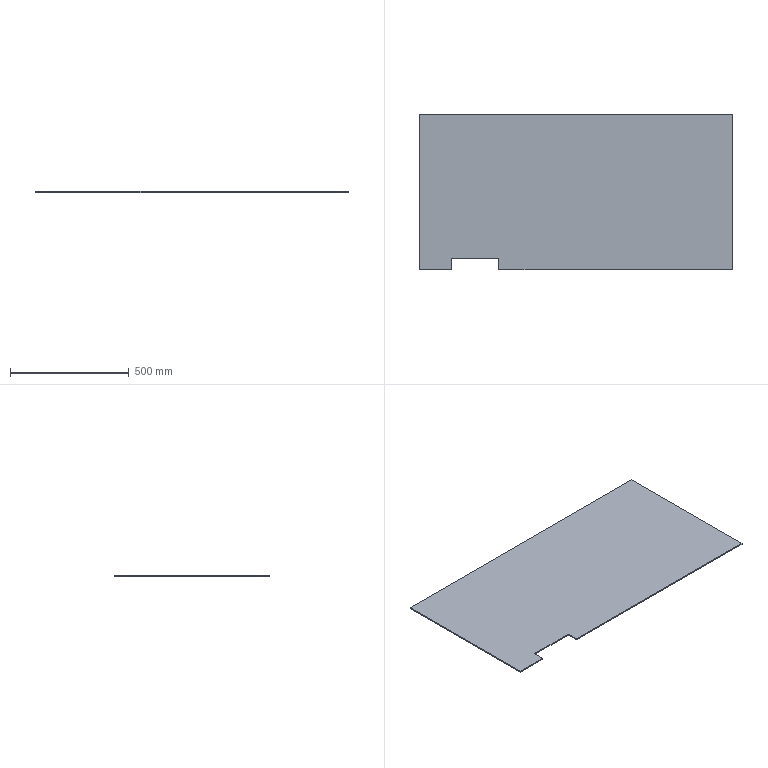Part | STEP file | 1 solid | 10 faces | box 1318 x 655 x 5 mm | volume 4267450 mm3 | plane 10
STEP:
#1=CARTESIAN_POINT('',(0.,0.,0.));
#2=DIRECTION('',(0.,0.,1.));
#3=DIRECTION('',(1.,0.,0.));
#4=AXIS2_PLACEMENT_3D('',#1,#2,#3);
#5=CARTESIAN_POINT('',(-324.,-657.,0.));
#6=VERTEX_POINT('',#5);
#7=CARTESIAN_POINT('',(-524.,-657.,0.));
#8=VERTEX_POINT('',#7);
#9=CARTESIAN_POINT('',(-524.,-657.,0.));
#10=DIRECTION('',(-1.,0.,0.));
#11=VECTOR('',#10,1.);
#12=LINE('',#9,#11);
#13=CARTESIAN_POINT('',(0.,0.,0.));
#14=DIRECTION('',(0.,0.,1.));
#15=DIRECTION('',(1.,0.,0.));
#16=AXIS2_PLACEMENT_3D('',#13,#14,#15);
#17=PLANE('',#16);
#18=CARTESIAN_POINT('',(-524.,-657.));
#19=DIRECTION('',(-1.,0.));
#20=VECTOR('',#19,1.);
#21=LINE('',#18,#20);
#22=(GEOMETRIC_REPRESENTATION_CONTEXT(2)PARAMETRIC_REPRESENTATION_CONTEXT()REPRESENTATION_CONTEXT('',''));
#23=DEFINITIONAL_REPRESENTATION('',(#21),#22);
#24=PCURVE('',#17,#23);
#25=CARTESIAN_POINT('',(-524.,-657.,5.));
#26=DIRECTION('',(0.,1.,0.));
#27=DIRECTION('',(1.,0.,0.));
#28=AXIS2_PLACEMENT_3D('',#25,#26,#27);
#29=PLANE('',#28);
#30=CARTESIAN_POINT('',(0.,5.));
#31=DIRECTION('',(-1.,0.));
#32=VECTOR('',#31,1.);
#33=LINE('',#30,#32);
#34=(GEOMETRIC_REPRESENTATION_CONTEXT(2)PARAMETRIC_REPRESENTATION_CONTEXT()REPRESENTATION_CONTEXT('',''));
#35=DEFINITIONAL_REPRESENTATION('',(#33),#34);
#36=PCURVE('',#29,#35);
#37=SURFACE_CURVE('',#12,(#24,#36),.PCURVE_S1.);
#38=EDGE_CURVE('',#6,#8,#37,.T.);
#39=ORIENTED_EDGE('',*,*,#38,.T.);
#40=CARTESIAN_POINT('',(-524.,-706.,0.));
#41=VERTEX_POINT('',#40);
#42=CARTESIAN_POINT('',(-524.,-657.,0.));
#43=DIRECTION('',(0.,1.,0.));
#44=VECTOR('',#43,1.);
#45=LINE('',#42,#44);
#46=CARTESIAN_POINT('',(-524.,-657.));
#47=DIRECTION('',(0.,1.));
#48=VECTOR('',#47,1.);
#49=LINE('',#46,#48);
#50=(GEOMETRIC_REPRESENTATION_CONTEXT(2)PARAMETRIC_REPRESENTATION_CONTEXT()REPRESENTATION_CONTEXT('',''));
#51=DEFINITIONAL_REPRESENTATION('',(#49),#50);
#52=PCURVE('',#17,#51);
#53=CARTESIAN_POINT('',(-524.,-657.,5.));
#54=DIRECTION('',(1.,0.,0.));
#55=DIRECTION('',(0.,1.,0.));
#56=AXIS2_PLACEMENT_3D('',#53,#54,#55);
#57=PLANE('',#56);
#58=CARTESIAN_POINT('',(0.,-5.));
#59=DIRECTION('',(1.,0.));
#60=VECTOR('',#59,1.);
#61=LINE('',#58,#60);
#62=(GEOMETRIC_REPRESENTATION_CONTEXT(2)PARAMETRIC_REPRESENTATION_CONTEXT()REPRESENTATION_CONTEXT('',''));
#63=DEFINITIONAL_REPRESENTATION('',(#61),#62);
#64=PCURVE('',#57,#63);
#65=SURFACE_CURVE('',#45,(#52,#64),.PCURVE_S1.);
#66=EDGE_CURVE('',#41,#8,#65,.T.);
#67=ORIENTED_EDGE('',*,*,#66,.F.);
#68=CARTESIAN_POINT('',(-659.,-706.,0.));
#69=VERTEX_POINT('',#68);
#70=CARTESIAN_POINT('',(-659.,-706.,0.));
#71=DIRECTION('',(-1.,0.,0.));
#72=VECTOR('',#71,1.);
#73=LINE('',#70,#72);
#74=CARTESIAN_POINT('',(-659.,-706.));
#75=DIRECTION('',(-1.,0.));
#76=VECTOR('',#75,1.);
#77=LINE('',#74,#76);
#78=(GEOMETRIC_REPRESENTATION_CONTEXT(2)PARAMETRIC_REPRESENTATION_CONTEXT()REPRESENTATION_CONTEXT('',''));
#79=DEFINITIONAL_REPRESENTATION('',(#77),#78);
#80=PCURVE('',#17,#79);
#81=CARTESIAN_POINT('',(-659.,-706.,5.));
#82=DIRECTION('',(0.,1.,0.));
#83=DIRECTION('',(1.,0.,0.));
#84=AXIS2_PLACEMENT_3D('',#81,#82,#83);
#85=PLANE('',#84);
#86=CARTESIAN_POINT('',(0.,5.));
#87=DIRECTION('',(-1.,0.));
#88=VECTOR('',#87,1.);
#89=LINE('',#86,#88);
#90=(GEOMETRIC_REPRESENTATION_CONTEXT(2)PARAMETRIC_REPRESENTATION_CONTEXT()REPRESENTATION_CONTEXT('',''));
#91=DEFINITIONAL_REPRESENTATION('',(#89),#90);
#92=PCURVE('',#85,#91);
#93=SURFACE_CURVE('',#73,(#80,#92),.PCURVE_S1.);
#94=EDGE_CURVE('',#41,#69,#93,.T.);
#95=ORIENTED_EDGE('',*,*,#94,.T.);
#96=CARTESIAN_POINT('',(-659.,-51.,0.));
#97=VERTEX_POINT('',#96);
#98=CARTESIAN_POINT('',(-659.,-51.,0.));
#99=DIRECTION('',(0.,1.,0.));
#100=VECTOR('',#99,1.);
#101=LINE('',#98,#100);
#102=CARTESIAN_POINT('',(-659.,-51.));
#103=DIRECTION('',(0.,1.));
#104=VECTOR('',#103,1.);
#105=LINE('',#102,#104);
#106=(GEOMETRIC_REPRESENTATION_CONTEXT(2)PARAMETRIC_REPRESENTATION_CONTEXT()REPRESENTATION_CONTEXT('',''));
#107=DEFINITIONAL_REPRESENTATION('',(#105),#106);
#108=PCURVE('',#17,#107);
#109=CARTESIAN_POINT('',(-659.,-51.,5.));
#110=DIRECTION('',(1.,0.,0.));
#111=DIRECTION('',(0.,1.,0.));
#112=AXIS2_PLACEMENT_3D('',#109,#110,#111);
#113=PLANE('',#112);
#114=CARTESIAN_POINT('',(0.,-5.));
#115=DIRECTION('',(1.,0.));
#116=VECTOR('',#115,1.);
#117=LINE('',#114,#116);
#118=(GEOMETRIC_REPRESENTATION_CONTEXT(2)PARAMETRIC_REPRESENTATION_CONTEXT()REPRESENTATION_CONTEXT('',''));
#119=DEFINITIONAL_REPRESENTATION('',(#117),#118);
#120=PCURVE('',#113,#119);
#121=SURFACE_CURVE('',#101,(#108,#120),.PCURVE_S1.);
#122=EDGE_CURVE('',#69,#97,#121,.T.);
#123=ORIENTED_EDGE('',*,*,#122,.T.);
#124=CARTESIAN_POINT('',(659.,-51.,0.));
#125=VERTEX_POINT('',#124);
#126=CARTESIAN_POINT('',(-659.,-51.,0.));
#127=DIRECTION('',(-1.,0.,0.));
#128=VECTOR('',#127,1.);
#129=LINE('',#126,#128);
#130=CARTESIAN_POINT('',(-659.,-51.));
#131=DIRECTION('',(-1.,0.));
#132=VECTOR('',#131,1.);
#133=LINE('',#130,#132);
#134=(GEOMETRIC_REPRESENTATION_CONTEXT(2)PARAMETRIC_REPRESENTATION_CONTEXT()REPRESENTATION_CONTEXT('',''));
#135=DEFINITIONAL_REPRESENTATION('',(#133),#134);
#136=PCURVE('',#17,#135);
#137=CARTESIAN_POINT('',(-659.,-51.,5.));
#138=DIRECTION('',(0.,1.,0.));
#139=DIRECTION('',(1.,0.,0.));
#140=AXIS2_PLACEMENT_3D('',#137,#138,#139);
#141=PLANE('',#140);
#142=CARTESIAN_POINT('',(0.,5.));
#143=DIRECTION('',(-1.,0.));
#144=VECTOR('',#143,1.);
#145=LINE('',#142,#144);
#146=(GEOMETRIC_REPRESENTATION_CONTEXT(2)PARAMETRIC_REPRESENTATION_CONTEXT()REPRESENTATION_CONTEXT('',''));
#147=DEFINITIONAL_REPRESENTATION('',(#145),#146);
#148=PCURVE('',#141,#147);
#149=SURFACE_CURVE('',#129,(#136,#148),.PCURVE_S1.);
#150=EDGE_CURVE('',#125,#97,#149,.T.);
#151=ORIENTED_EDGE('',*,*,#150,.F.);
#152=CARTESIAN_POINT('',(659.,-706.,0.));
#153=VERTEX_POINT('',#152);
#154=CARTESIAN_POINT('',(659.,-51.,0.));
#155=DIRECTION('',(0.,1.,0.));
#156=VECTOR('',#155,1.);
#157=LINE('',#154,#156);
#158=CARTESIAN_POINT('',(659.,-51.));
#159=DIRECTION('',(0.,1.));
#160=VECTOR('',#159,1.);
#161=LINE('',#158,#160);
#162=(GEOMETRIC_REPRESENTATION_CONTEXT(2)PARAMETRIC_REPRESENTATION_CONTEXT()REPRESENTATION_CONTEXT('',''));
#163=DEFINITIONAL_REPRESENTATION('',(#161),#162);
#164=PCURVE('',#17,#163);
#165=CARTESIAN_POINT('',(659.,-51.,5.));
#166=DIRECTION('',(1.,0.,0.));
#167=DIRECTION('',(0.,1.,0.));
#168=AXIS2_PLACEMENT_3D('',#165,#166,#167);
#169=PLANE('',#168);
#170=CARTESIAN_POINT('',(0.,-5.));
#171=DIRECTION('',(1.,0.));
#172=VECTOR('',#171,1.);
#173=LINE('',#170,#172);
#174=(GEOMETRIC_REPRESENTATION_CONTEXT(2)PARAMETRIC_REPRESENTATION_CONTEXT()REPRESENTATION_CONTEXT('',''));
#175=DEFINITIONAL_REPRESENTATION('',(#173),#174);
#176=PCURVE('',#169,#175);
#177=SURFACE_CURVE('',#157,(#164,#176),.PCURVE_S1.);
#178=EDGE_CURVE('',#153,#125,#177,.T.);
#179=ORIENTED_EDGE('',*,*,#178,.F.);
#180=CARTESIAN_POINT('',(-324.,-706.,0.));
#181=VERTEX_POINT('',#180);
#182=CARTESIAN_POINT('',(-324.,-706.,0.));
#183=DIRECTION('',(-1.,0.,0.));
#184=VECTOR('',#183,1.);
#185=LINE('',#182,#184);
#186=CARTESIAN_POINT('',(-324.,-706.));
#187=DIRECTION('',(-1.,0.));
#188=VECTOR('',#187,1.);
#189=LINE('',#186,#188);
#190=(GEOMETRIC_REPRESENTATION_CONTEXT(2)PARAMETRIC_REPRESENTATION_CONTEXT()REPRESENTATION_CONTEXT('',''));
#191=DEFINITIONAL_REPRESENTATION('',(#189),#190);
#192=PCURVE('',#17,#191);
#193=CARTESIAN_POINT('',(-324.,-706.,5.));
#194=DIRECTION('',(0.,1.,0.));
#195=DIRECTION('',(1.,0.,0.));
#196=AXIS2_PLACEMENT_3D('',#193,#194,#195);
#197=PLANE('',#196);
#198=CARTESIAN_POINT('',(0.,5.));
#199=DIRECTION('',(-1.,0.));
#200=VECTOR('',#199,1.);
#201=LINE('',#198,#200);
#202=(GEOMETRIC_REPRESENTATION_CONTEXT(2)PARAMETRIC_REPRESENTATION_CONTEXT()REPRESENTATION_CONTEXT('',''));
#203=DEFINITIONAL_REPRESENTATION('',(#201),#202);
#204=PCURVE('',#197,#203);
#205=SURFACE_CURVE('',#185,(#192,#204),.PCURVE_S1.);
#206=EDGE_CURVE('',#153,#181,#205,.T.);
#207=ORIENTED_EDGE('',*,*,#206,.T.);
#208=CARTESIAN_POINT('',(-324.,-657.,0.));
#209=DIRECTION('',(0.,1.,0.));
#210=VECTOR('',#209,1.);
#211=LINE('',#208,#210);
#212=CARTESIAN_POINT('',(-324.,-657.));
#213=DIRECTION('',(0.,1.));
#214=VECTOR('',#213,1.);
#215=LINE('',#212,#214);
#216=(GEOMETRIC_REPRESENTATION_CONTEXT(2)PARAMETRIC_REPRESENTATION_CONTEXT()REPRESENTATION_CONTEXT('',''));
#217=DEFINITIONAL_REPRESENTATION('',(#215),#216);
#218=PCURVE('',#17,#217);
#219=CARTESIAN_POINT('',(-324.,-657.,5.));
#220=DIRECTION('',(1.,0.,0.));
#221=DIRECTION('',(0.,-1.,0.));
#222=AXIS2_PLACEMENT_3D('',#219,#220,#221);
#223=PLANE('',#222);
#224=CARTESIAN_POINT('',(0.,5.));
#225=DIRECTION('',(-1.,0.));
#226=VECTOR('',#225,1.);
#227=LINE('',#224,#226);
#228=(GEOMETRIC_REPRESENTATION_CONTEXT(2)PARAMETRIC_REPRESENTATION_CONTEXT()REPRESENTATION_CONTEXT('',''));
#229=DEFINITIONAL_REPRESENTATION('',(#227),#228);
#230=PCURVE('',#223,#229);
#231=SURFACE_CURVE('',#211,(#218,#230),.PCURVE_S1.);
#232=EDGE_CURVE('',#181,#6,#231,.T.);
#233=ORIENTED_EDGE('',*,*,#232,.T.);
#234=EDGE_LOOP('',(#39,#67,#95,#123,#151,#179,#207,#233));
#235=FACE_BOUND('',#234,.T.);
#236=ADVANCED_FACE('',(#235),#17,.F.);
#237=CARTESIAN_POINT('',(-324.,-706.,5.));
#238=VERTEX_POINT('',#237);
#239=CARTESIAN_POINT('',(-324.,-706.,5.));
#240=DIRECTION('',(0.,0.,1.));
#241=VECTOR('',#240,1.);
#242=LINE('',#239,#241);
#243=CARTESIAN_POINT('',(49.,0.));
#244=DIRECTION('',(0.,-1.));
#245=VECTOR('',#244,1.);
#246=LINE('',#243,#245);
#247=(GEOMETRIC_REPRESENTATION_CONTEXT(2)PARAMETRIC_REPRESENTATION_CONTEXT()REPRESENTATION_CONTEXT('',''));
#248=DEFINITIONAL_REPRESENTATION('',(#246),#247);
#249=PCURVE('',#223,#248);
#250=CARTESIAN_POINT('',(0.,0.));
#251=DIRECTION('',(0.,-1.));
#252=VECTOR('',#251,1.);
#253=LINE('',#250,#252);
#254=(GEOMETRIC_REPRESENTATION_CONTEXT(2)PARAMETRIC_REPRESENTATION_CONTEXT()REPRESENTATION_CONTEXT('',''));
#255=DEFINITIONAL_REPRESENTATION('',(#253),#254);
#256=PCURVE('',#197,#255);
#257=SURFACE_CURVE('',#242,(#249,#256),.PCURVE_S1.);
#258=EDGE_CURVE('',#181,#238,#257,.T.);
#259=ORIENTED_EDGE('',*,*,#258,.T.);
#260=CARTESIAN_POINT('',(-324.,-657.,5.));
#261=VERTEX_POINT('',#260);
#262=CARTESIAN_POINT('',(-324.,0.,5.));
#263=DIRECTION('',(0.,-1.,0.));
#264=VECTOR('',#263,1.);
#265=LINE('',#262,#264);
#266=CARTESIAN_POINT('',(-657.,0.));
#267=DIRECTION('',(1.,0.));
#268=VECTOR('',#267,1.);
#269=LINE('',#266,#268);
#270=(GEOMETRIC_REPRESENTATION_CONTEXT(2)PARAMETRIC_REPRESENTATION_CONTEXT()REPRESENTATION_CONTEXT('',''));
#271=DEFINITIONAL_REPRESENTATION('',(#269),#270);
#272=PCURVE('',#223,#271);
#273=CARTESIAN_POINT('',(0.,0.,5.));
#274=DIRECTION('',(0.,0.,1.));
#275=DIRECTION('',(1.,0.,0.));
#276=AXIS2_PLACEMENT_3D('',#273,#274,#275);
#277=PLANE('',#276);
#278=CARTESIAN_POINT('',(-324.,0.));
#279=DIRECTION('',(0.,-1.));
#280=VECTOR('',#279,1.);
#281=LINE('',#278,#280);
#282=(GEOMETRIC_REPRESENTATION_CONTEXT(2)PARAMETRIC_REPRESENTATION_CONTEXT()REPRESENTATION_CONTEXT('',''));
#283=DEFINITIONAL_REPRESENTATION('',(#281),#282);
#284=PCURVE('',#277,#283);
#285=SURFACE_CURVE('',#265,(#272,#284),.PCURVE_S1.);
#286=EDGE_CURVE('',#261,#238,#285,.T.);
#287=ORIENTED_EDGE('',*,*,#286,.F.);
#288=CARTESIAN_POINT('',(-324.,-657.,5.));
#289=DIRECTION('',(0.,0.,-1.));
#290=VECTOR('',#289,1.);
#291=LINE('',#288,#290);
#292=CARTESIAN_POINT('',(0.,0.));
#293=DIRECTION('',(0.,1.));
#294=VECTOR('',#293,1.);
#295=LINE('',#292,#294);
#296=(GEOMETRIC_REPRESENTATION_CONTEXT(2)PARAMETRIC_REPRESENTATION_CONTEXT()REPRESENTATION_CONTEXT('',''));
#297=DEFINITIONAL_REPRESENTATION('',(#295),#296);
#298=PCURVE('',#223,#297);
#299=CARTESIAN_POINT('',(200.,0.));
#300=DIRECTION('',(0.,1.));
#301=VECTOR('',#300,1.);
#302=LINE('',#299,#301);
#303=(GEOMETRIC_REPRESENTATION_CONTEXT(2)PARAMETRIC_REPRESENTATION_CONTEXT()REPRESENTATION_CONTEXT('',''));
#304=DEFINITIONAL_REPRESENTATION('',(#302),#303);
#305=PCURVE('',#29,#304);
#306=SURFACE_CURVE('',#291,(#298,#305),.PCURVE_S1.);
#307=EDGE_CURVE('',#261,#6,#306,.T.);
#308=ORIENTED_EDGE('',*,*,#307,.T.);
#309=ORIENTED_EDGE('',*,*,#232,.F.);
#310=EDGE_LOOP('',(#259,#287,#308,#309));
#311=FACE_BOUND('',#310,.T.);
#312=ADVANCED_FACE('',(#311),#223,.F.);
#313=CARTESIAN_POINT('',(659.,-706.,5.));
#314=VERTEX_POINT('',#313);
#315=CARTESIAN_POINT('',(659.,-706.,5.));
#316=DIRECTION('',(0.,0.,-1.));
#317=VECTOR('',#316,1.);
#318=LINE('',#315,#317);
#319=CARTESIAN_POINT('',(983.,0.));
#320=DIRECTION('',(0.,1.));
#321=VECTOR('',#320,1.);
#322=LINE('',#319,#321);
#323=(GEOMETRIC_REPRESENTATION_CONTEXT(2)PARAMETRIC_REPRESENTATION_CONTEXT()REPRESENTATION_CONTEXT('',''));
#324=DEFINITIONAL_REPRESENTATION('',(#322),#323);
#325=PCURVE('',#197,#324);
#326=CARTESIAN_POINT('',(-655.,0.));
#327=DIRECTION('',(0.,-1.));
#328=VECTOR('',#327,1.);
#329=LINE('',#326,#328);
#330=(GEOMETRIC_REPRESENTATION_CONTEXT(2)PARAMETRIC_REPRESENTATION_CONTEXT()REPRESENTATION_CONTEXT('',''));
#331=DEFINITIONAL_REPRESENTATION('',(#329),#330);
#332=PCURVE('',#169,#331);
#333=SURFACE_CURVE('',#318,(#325,#332),.PCURVE_S1.);
#334=EDGE_CURVE('',#314,#153,#333,.T.);
#335=ORIENTED_EDGE('',*,*,#334,.F.);
#336=CARTESIAN_POINT('',(0.,-706.,5.));
#337=DIRECTION('',(1.,0.,0.));
#338=VECTOR('',#337,1.);
#339=LINE('',#336,#338);
#340=CARTESIAN_POINT('',(324.,0.));
#341=DIRECTION('',(1.,0.));
#342=VECTOR('',#341,1.);
#343=LINE('',#340,#342);
#344=(GEOMETRIC_REPRESENTATION_CONTEXT(2)PARAMETRIC_REPRESENTATION_CONTEXT()REPRESENTATION_CONTEXT('',''));
#345=DEFINITIONAL_REPRESENTATION('',(#343),#344);
#346=PCURVE('',#197,#345);
#347=CARTESIAN_POINT('',(0.,-706.));
#348=DIRECTION('',(1.,0.));
#349=VECTOR('',#348,1.);
#350=LINE('',#347,#349);
#351=(GEOMETRIC_REPRESENTATION_CONTEXT(2)PARAMETRIC_REPRESENTATION_CONTEXT()REPRESENTATION_CONTEXT('',''));
#352=DEFINITIONAL_REPRESENTATION('',(#350),#351);
#353=PCURVE('',#277,#352);
#354=SURFACE_CURVE('',#339,(#346,#353),.PCURVE_S1.);
#355=EDGE_CURVE('',#238,#314,#354,.T.);
#356=ORIENTED_EDGE('',*,*,#355,.F.);
#357=ORIENTED_EDGE('',*,*,#258,.F.);
#358=ORIENTED_EDGE('',*,*,#206,.F.);
#359=EDGE_LOOP('',(#335,#356,#357,#358));
#360=FACE_BOUND('',#359,.T.);
#361=ADVANCED_FACE('',(#360),#197,.F.);
#362=CARTESIAN_POINT('',(659.,-51.,5.));
#363=VERTEX_POINT('',#362);
#364=CARTESIAN_POINT('',(659.,0.,5.));
#365=DIRECTION('',(0.,1.,0.));
#366=VECTOR('',#365,1.);
#367=LINE('',#364,#366);
#368=CARTESIAN_POINT('',(51.,0.));
#369=DIRECTION('',(1.,0.));
#370=VECTOR('',#369,1.);
#371=LINE('',#368,#370);
#372=(GEOMETRIC_REPRESENTATION_CONTEXT(2)PARAMETRIC_REPRESENTATION_CONTEXT()REPRESENTATION_CONTEXT('',''));
#373=DEFINITIONAL_REPRESENTATION('',(#371),#372);
#374=PCURVE('',#169,#373);
#375=CARTESIAN_POINT('',(659.,0.));
#376=DIRECTION('',(0.,1.));
#377=VECTOR('',#376,1.);
#378=LINE('',#375,#377);
#379=(GEOMETRIC_REPRESENTATION_CONTEXT(2)PARAMETRIC_REPRESENTATION_CONTEXT()REPRESENTATION_CONTEXT('',''));
#380=DEFINITIONAL_REPRESENTATION('',(#378),#379);
#381=PCURVE('',#277,#380);
#382=SURFACE_CURVE('',#367,(#374,#381),.PCURVE_S1.);
#383=EDGE_CURVE('',#314,#363,#382,.T.);
#384=ORIENTED_EDGE('',*,*,#383,.F.);
#385=ORIENTED_EDGE('',*,*,#334,.T.);
#386=ORIENTED_EDGE('',*,*,#178,.T.);
#387=CARTESIAN_POINT('',(659.,-51.,5.));
#388=DIRECTION('',(0.,0.,-1.));
#389=VECTOR('',#388,1.);
#390=LINE('',#387,#389);
#391=CARTESIAN_POINT('',(0.,0.));
#392=DIRECTION('',(0.,-1.));
#393=VECTOR('',#392,1.);
#394=LINE('',#391,#393);
#395=(GEOMETRIC_REPRESENTATION_CONTEXT(2)PARAMETRIC_REPRESENTATION_CONTEXT()REPRESENTATION_CONTEXT('',''));
#396=DEFINITIONAL_REPRESENTATION('',(#394),#395);
#397=PCURVE('',#169,#396);
#398=CARTESIAN_POINT('',(1318.,0.));
#399=DIRECTION('',(0.,1.));
#400=VECTOR('',#399,1.);
#401=LINE('',#398,#400);
#402=(GEOMETRIC_REPRESENTATION_CONTEXT(2)PARAMETRIC_REPRESENTATION_CONTEXT()REPRESENTATION_CONTEXT('',''));
#403=DEFINITIONAL_REPRESENTATION('',(#401),#402);
#404=PCURVE('',#141,#403);
#405=SURFACE_CURVE('',#390,(#397,#404),.PCURVE_S1.);
#406=EDGE_CURVE('',#363,#125,#405,.T.);
#407=ORIENTED_EDGE('',*,*,#406,.F.);
#408=EDGE_LOOP('',(#384,#385,#386,#407));
#409=FACE_BOUND('',#408,.T.);
#410=ADVANCED_FACE('',(#409),#169,.T.);
#411=CARTESIAN_POINT('',(-659.,-51.,5.));
#412=VERTEX_POINT('',#411);
#413=CARTESIAN_POINT('',(0.,-51.,5.));
#414=DIRECTION('',(-1.,0.,0.));
#415=VECTOR('',#414,1.);
#416=LINE('',#413,#415);
#417=CARTESIAN_POINT('',(659.,0.));
#418=DIRECTION('',(-1.,0.));
#419=VECTOR('',#418,1.);
#420=LINE('',#417,#419);
#421=(GEOMETRIC_REPRESENTATION_CONTEXT(2)PARAMETRIC_REPRESENTATION_CONTEXT()REPRESENTATION_CONTEXT('',''));
#422=DEFINITIONAL_REPRESENTATION('',(#420),#421);
#423=PCURVE('',#141,#422);
#424=CARTESIAN_POINT('',(0.,-51.));
#425=DIRECTION('',(-1.,0.));
#426=VECTOR('',#425,1.);
#427=LINE('',#424,#426);
#428=(GEOMETRIC_REPRESENTATION_CONTEXT(2)PARAMETRIC_REPRESENTATION_CONTEXT()REPRESENTATION_CONTEXT('',''));
#429=DEFINITIONAL_REPRESENTATION('',(#427),#428);
#430=PCURVE('',#277,#429);
#431=SURFACE_CURVE('',#416,(#423,#430),.PCURVE_S1.);
#432=EDGE_CURVE('',#363,#412,#431,.T.);
#433=ORIENTED_EDGE('',*,*,#432,.F.);
#434=ORIENTED_EDGE('',*,*,#406,.T.);
#435=ORIENTED_EDGE('',*,*,#150,.T.);
#436=CARTESIAN_POINT('',(-659.,-51.,5.));
#437=DIRECTION('',(0.,0.,1.));
#438=VECTOR('',#437,1.);
#439=LINE('',#436,#438);
#440=CARTESIAN_POINT('',(0.,0.));
#441=DIRECTION('',(0.,-1.));
#442=VECTOR('',#441,1.);
#443=LINE('',#440,#442);
#444=(GEOMETRIC_REPRESENTATION_CONTEXT(2)PARAMETRIC_REPRESENTATION_CONTEXT()REPRESENTATION_CONTEXT('',''));
#445=DEFINITIONAL_REPRESENTATION('',(#443),#444);
#446=PCURVE('',#141,#445);
#447=CARTESIAN_POINT('',(0.,0.));
#448=DIRECTION('',(0.,1.));
#449=VECTOR('',#448,1.);
#450=LINE('',#447,#449);
#451=(GEOMETRIC_REPRESENTATION_CONTEXT(2)PARAMETRIC_REPRESENTATION_CONTEXT()REPRESENTATION_CONTEXT('',''));
#452=DEFINITIONAL_REPRESENTATION('',(#450),#451);
#453=PCURVE('',#113,#452);
#454=SURFACE_CURVE('',#439,(#446,#453),.PCURVE_S1.);
#455=EDGE_CURVE('',#97,#412,#454,.T.);
#456=ORIENTED_EDGE('',*,*,#455,.T.);
#457=EDGE_LOOP('',(#433,#434,#435,#456));
#458=FACE_BOUND('',#457,.T.);
#459=ADVANCED_FACE('',(#458),#141,.T.);
#460=CARTESIAN_POINT('',(-659.,-706.,5.));
#461=VERTEX_POINT('',#460);
#462=CARTESIAN_POINT('',(-659.,-706.,5.));
#463=DIRECTION('',(0.,0.,1.));
#464=VECTOR('',#463,1.);
#465=LINE('',#462,#464);
#466=CARTESIAN_POINT('',(-655.,0.));
#467=DIRECTION('',(0.,1.));
#468=VECTOR('',#467,1.);
#469=LINE('',#466,#468);
#470=(GEOMETRIC_REPRESENTATION_CONTEXT(2)PARAMETRIC_REPRESENTATION_CONTEXT()REPRESENTATION_CONTEXT('',''));
#471=DEFINITIONAL_REPRESENTATION('',(#469),#470);
#472=PCURVE('',#113,#471);
#473=CARTESIAN_POINT('',(0.,0.));
#474=DIRECTION('',(0.,-1.));
#475=VECTOR('',#474,1.);
#476=LINE('',#473,#475);
#477=(GEOMETRIC_REPRESENTATION_CONTEXT(2)PARAMETRIC_REPRESENTATION_CONTEXT()REPRESENTATION_CONTEXT('',''));
#478=DEFINITIONAL_REPRESENTATION('',(#476),#477);
#479=PCURVE('',#85,#478);
#480=SURFACE_CURVE('',#465,(#472,#479),.PCURVE_S1.);
#481=EDGE_CURVE('',#69,#461,#480,.T.);
#482=ORIENTED_EDGE('',*,*,#481,.T.);
#483=CARTESIAN_POINT('',(-659.,0.,5.));
#484=DIRECTION('',(0.,-1.,0.));
#485=VECTOR('',#484,1.);
#486=LINE('',#483,#485);
#487=CARTESIAN_POINT('',(51.,0.));
#488=DIRECTION('',(-1.,0.));
#489=VECTOR('',#488,1.);
#490=LINE('',#487,#489);
#491=(GEOMETRIC_REPRESENTATION_CONTEXT(2)PARAMETRIC_REPRESENTATION_CONTEXT()REPRESENTATION_CONTEXT('',''));
#492=DEFINITIONAL_REPRESENTATION('',(#490),#491);
#493=PCURVE('',#113,#492);
#494=CARTESIAN_POINT('',(-659.,0.));
#495=DIRECTION('',(0.,-1.));
#496=VECTOR('',#495,1.);
#497=LINE('',#494,#496);
#498=(GEOMETRIC_REPRESENTATION_CONTEXT(2)PARAMETRIC_REPRESENTATION_CONTEXT()REPRESENTATION_CONTEXT('',''));
#499=DEFINITIONAL_REPRESENTATION('',(#497),#498);
#500=PCURVE('',#277,#499);
#501=SURFACE_CURVE('',#486,(#493,#500),.PCURVE_S1.);
#502=EDGE_CURVE('',#412,#461,#501,.T.);
#503=ORIENTED_EDGE('',*,*,#502,.F.);
#504=ORIENTED_EDGE('',*,*,#455,.F.);
#505=ORIENTED_EDGE('',*,*,#122,.F.);
#506=EDGE_LOOP('',(#482,#503,#504,#505));
#507=FACE_BOUND('',#506,.T.);
#508=ADVANCED_FACE('',(#507),#113,.F.);
#509=CARTESIAN_POINT('',(-524.,-706.,5.));
#510=VERTEX_POINT('',#509);
#511=CARTESIAN_POINT('',(-524.,-706.,5.));
#512=DIRECTION('',(0.,0.,-1.));
#513=VECTOR('',#512,1.);
#514=LINE('',#511,#513);
#515=CARTESIAN_POINT('',(135.,0.));
#516=DIRECTION('',(0.,1.));
#517=VECTOR('',#516,1.);
#518=LINE('',#515,#517);
#519=(GEOMETRIC_REPRESENTATION_CONTEXT(2)PARAMETRIC_REPRESENTATION_CONTEXT()REPRESENTATION_CONTEXT('',''));
#520=DEFINITIONAL_REPRESENTATION('',(#518),#519);
#521=PCURVE('',#85,#520);
#522=CARTESIAN_POINT('',(-49.,0.));
#523=DIRECTION('',(0.,-1.));
#524=VECTOR('',#523,1.);
#525=LINE('',#522,#524);
#526=(GEOMETRIC_REPRESENTATION_CONTEXT(2)PARAMETRIC_REPRESENTATION_CONTEXT()REPRESENTATION_CONTEXT('',''));
#527=DEFINITIONAL_REPRESENTATION('',(#525),#526);
#528=PCURVE('',#57,#527);
#529=SURFACE_CURVE('',#514,(#521,#528),.PCURVE_S1.);
#530=EDGE_CURVE('',#510,#41,#529,.T.);
#531=ORIENTED_EDGE('',*,*,#530,.F.);
#532=CARTESIAN_POINT('',(0.,-706.,5.));
#533=DIRECTION('',(1.,0.,0.));
#534=VECTOR('',#533,1.);
#535=LINE('',#532,#534);
#536=CARTESIAN_POINT('',(659.,0.));
#537=DIRECTION('',(1.,0.));
#538=VECTOR('',#537,1.);
#539=LINE('',#536,#538);
#540=(GEOMETRIC_REPRESENTATION_CONTEXT(2)PARAMETRIC_REPRESENTATION_CONTEXT()REPRESENTATION_CONTEXT('',''));
#541=DEFINITIONAL_REPRESENTATION('',(#539),#540);
#542=PCURVE('',#85,#541);
#543=CARTESIAN_POINT('',(0.,-706.));
#544=DIRECTION('',(1.,0.));
#545=VECTOR('',#544,1.);
#546=LINE('',#543,#545);
#547=(GEOMETRIC_REPRESENTATION_CONTEXT(2)PARAMETRIC_REPRESENTATION_CONTEXT()REPRESENTATION_CONTEXT('',''));
#548=DEFINITIONAL_REPRESENTATION('',(#546),#547);
#549=PCURVE('',#277,#548);
#550=SURFACE_CURVE('',#535,(#542,#549),.PCURVE_S1.);
#551=EDGE_CURVE('',#461,#510,#550,.T.);
#552=ORIENTED_EDGE('',*,*,#551,.F.);
#553=ORIENTED_EDGE('',*,*,#481,.F.);
#554=ORIENTED_EDGE('',*,*,#94,.F.);
#555=EDGE_LOOP('',(#531,#552,#553,#554));
#556=FACE_BOUND('',#555,.T.);
#557=ADVANCED_FACE('',(#556),#85,.F.);
#558=CARTESIAN_POINT('',(-524.,-657.,5.));
#559=VERTEX_POINT('',#558);
#560=CARTESIAN_POINT('',(-524.,0.,5.));
#561=DIRECTION('',(0.,1.,0.));
#562=VECTOR('',#561,1.);
#563=LINE('',#560,#562);
#564=CARTESIAN_POINT('',(657.,0.));
#565=DIRECTION('',(1.,0.));
#566=VECTOR('',#565,1.);
#567=LINE('',#564,#566);
#568=(GEOMETRIC_REPRESENTATION_CONTEXT(2)PARAMETRIC_REPRESENTATION_CONTEXT()REPRESENTATION_CONTEXT('',''));
#569=DEFINITIONAL_REPRESENTATION('',(#567),#568);
#570=PCURVE('',#57,#569);
#571=CARTESIAN_POINT('',(-524.,0.));
#572=DIRECTION('',(0.,1.));
#573=VECTOR('',#572,1.);
#574=LINE('',#571,#573);
#575=(GEOMETRIC_REPRESENTATION_CONTEXT(2)PARAMETRIC_REPRESENTATION_CONTEXT()REPRESENTATION_CONTEXT('',''));
#576=DEFINITIONAL_REPRESENTATION('',(#574),#575);
#577=PCURVE('',#277,#576);
#578=SURFACE_CURVE('',#563,(#570,#577),.PCURVE_S1.);
#579=EDGE_CURVE('',#510,#559,#578,.T.);
#580=ORIENTED_EDGE('',*,*,#579,.F.);
#581=ORIENTED_EDGE('',*,*,#530,.T.);
#582=ORIENTED_EDGE('',*,*,#66,.T.);
#583=CARTESIAN_POINT('',(-524.,-657.,5.));
#584=DIRECTION('',(0.,0.,1.));
#585=VECTOR('',#584,1.);
#586=LINE('',#583,#585);
#587=CARTESIAN_POINT('',(0.,0.));
#588=DIRECTION('',(0.,1.));
#589=VECTOR('',#588,1.);
#590=LINE('',#587,#589);
#591=(GEOMETRIC_REPRESENTATION_CONTEXT(2)PARAMETRIC_REPRESENTATION_CONTEXT()REPRESENTATION_CONTEXT('',''));
#592=DEFINITIONAL_REPRESENTATION('',(#590),#591);
#593=PCURVE('',#57,#592);
#594=CARTESIAN_POINT('',(0.,0.));
#595=DIRECTION('',(0.,-1.));
#596=VECTOR('',#595,1.);
#597=LINE('',#594,#596);
#598=(GEOMETRIC_REPRESENTATION_CONTEXT(2)PARAMETRIC_REPRESENTATION_CONTEXT()REPRESENTATION_CONTEXT('',''));
#599=DEFINITIONAL_REPRESENTATION('',(#597),#598);
#600=PCURVE('',#29,#599);
#601=SURFACE_CURVE('',#586,(#593,#600),.PCURVE_S1.);
#602=EDGE_CURVE('',#8,#559,#601,.T.);
#603=ORIENTED_EDGE('',*,*,#602,.T.);
#604=EDGE_LOOP('',(#580,#581,#582,#603));
#605=FACE_BOUND('',#604,.T.);
#606=ADVANCED_FACE('',(#605),#57,.T.);
#607=ORIENTED_EDGE('',*,*,#307,.F.);
#608=CARTESIAN_POINT('',(0.,-657.,5.));
#609=DIRECTION('',(1.,0.,0.));
#610=VECTOR('',#609,1.);
#611=LINE('',#608,#610);
#612=CARTESIAN_POINT('',(524.,0.));
#613=DIRECTION('',(1.,0.));
#614=VECTOR('',#613,1.);
#615=LINE('',#612,#614);
#616=(GEOMETRIC_REPRESENTATION_CONTEXT(2)PARAMETRIC_REPRESENTATION_CONTEXT()REPRESENTATION_CONTEXT('',''));
#617=DEFINITIONAL_REPRESENTATION('',(#615),#616);
#618=PCURVE('',#29,#617);
#619=CARTESIAN_POINT('',(0.,-657.));
#620=DIRECTION('',(1.,0.));
#621=VECTOR('',#620,1.);
#622=LINE('',#619,#621);
#623=(GEOMETRIC_REPRESENTATION_CONTEXT(2)PARAMETRIC_REPRESENTATION_CONTEXT()REPRESENTATION_CONTEXT('',''));
#624=DEFINITIONAL_REPRESENTATION('',(#622),#623);
#625=PCURVE('',#277,#624);
#626=SURFACE_CURVE('',#611,(#618,#625),.PCURVE_S1.);
#627=EDGE_CURVE('',#559,#261,#626,.T.);
#628=ORIENTED_EDGE('',*,*,#627,.F.);
#629=ORIENTED_EDGE('',*,*,#602,.F.);
#630=ORIENTED_EDGE('',*,*,#38,.F.);
#631=EDGE_LOOP('',(#607,#628,#629,#630));
#632=FACE_BOUND('',#631,.T.);
#633=ADVANCED_FACE('',(#632),#29,.F.);
#634=ORIENTED_EDGE('',*,*,#579,.T.);
#635=ORIENTED_EDGE('',*,*,#627,.T.);
#636=ORIENTED_EDGE('',*,*,#286,.T.);
#637=ORIENTED_EDGE('',*,*,#355,.T.);
#638=ORIENTED_EDGE('',*,*,#383,.T.);
#639=ORIENTED_EDGE('',*,*,#432,.T.);
#640=ORIENTED_EDGE('',*,*,#502,.T.);
#641=ORIENTED_EDGE('',*,*,#551,.T.);
#642=EDGE_LOOP('',(#634,#635,#636,#637,#638,#639,#640,#641));
#643=FACE_BOUND('',#642,.T.);
#644=ADVANCED_FACE('',(#643),#277,.T.);
#645=CLOSED_SHELL('',(#236,#312,#361,#410,#459,#508,#557,#606,#633,#644));
#646=MANIFOLD_SOLID_BREP('',#645);
#647=(LENGTH_UNIT()NAMED_UNIT(*)SI_UNIT(.MILLI.,.METRE.));
#648=UNCERTAINTY_MEASURE_WITH_UNIT(LENGTH_MEASURE(0.0000001),#647,'','');
#649=(NAMED_UNIT(*)PLANE_ANGLE_UNIT()SI_UNIT($,.RADIAN.));
#650=(NAMED_UNIT(*)SI_UNIT($,.STERADIAN.)SOLID_ANGLE_UNIT());
#651=(GEOMETRIC_REPRESENTATION_CONTEXT(3)GLOBAL_UNCERTAINTY_ASSIGNED_CONTEXT((#648))GLOBAL_UNIT_ASSIGNED_CONTEXT((#647,#649,#650))REPRESENTATION_CONTEXT('',''));
#652=ADVANCED_BREP_SHAPE_REPRESENTATION('',(#4,#646),#651);